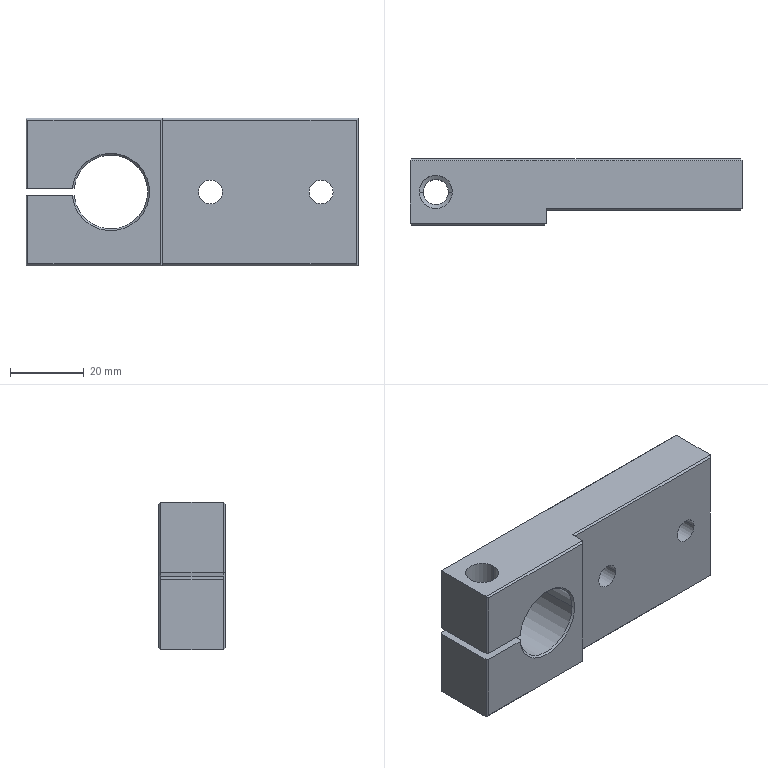Part | NX | 1 solid | 45 faces | box 90 x 18 x 40 mm | volume 46471 mm3 | plane 26 | cylinder 14 | cone 5 | commonest cylinder face diameters 6.5 x4 11 x4 6.8 x2 9 x2 20 x2
STEP:
#1=CARTESIAN_POINT('',(0.,17.5,-15.));
#2=VERTEX_POINT('',#1);
#3=CARTESIAN_POINT('',(0.5,18.,-14.5));
#4=VERTEX_POINT('',#3);
#5=CARTESIAN_POINT('',(15.,32.5,0.));
#6=DIRECTION('',(0.5774,0.5774,0.5774));
#7=VECTOR('',#6,1000.);
#8=LINE('',#5,#7);
#9=EDGE_CURVE('',#2,#4,#8,.T.);
#10=ORIENTED_EDGE('',*,*,#9,.F.);
#11=CARTESIAN_POINT('',(0.,17.5,4.));
#12=VERTEX_POINT('',#11);
#13=CARTESIAN_POINT('',(0.,17.5,0.));
#14=DIRECTION('',(0.,0.,-1.));
#15=VECTOR('',#14,1000.);
#16=LINE('',#13,#15);
#17=EDGE_CURVE('',#12,#2,#16,.T.);
#18=ORIENTED_EDGE('',*,*,#17,.F.);
#19=CARTESIAN_POINT('',(0.5,18.,4.));
#20=VERTEX_POINT('',#19);
#21=CARTESIAN_POINT('',(-17.5,0.,4.));
#22=DIRECTION('',(0.7071,0.7071,0.));
#23=VECTOR('',#22,1000.);
#24=LINE('',#21,#23);
#25=EDGE_CURVE('',#12,#20,#24,.T.);
#26=ORIENTED_EDGE('',*,*,#25,.T.);
#27=CARTESIAN_POINT('',(0.5,18.,0.));
#28=DIRECTION('',(0.,0.,-1.));
#29=VECTOR('',#28,1000.);
#30=LINE('',#27,#29);
#31=EDGE_CURVE('',#20,#4,#30,.T.);
#32=ORIENTED_EDGE('',*,*,#31,.T.);
#33=EDGE_LOOP('',(#10,#18,#26,#32));
#34=FACE_BOUND('',#33,.T.);
#35=CARTESIAN_POINT('',(0.,17.5,-16.5));
#36=DIRECTION('',(-0.7071,0.7071,0.));
#37=DIRECTION('',(0.,0.,1.));
#38=AXIS2_PLACEMENT_3D('',#35,#36,#37);
#39=PLANE('',#38);
#40=ADVANCED_FACE('',(#34),#39,.T.);
#41=CARTESIAN_POINT('',(37.,0.5,-15.));
#42=VERTEX_POINT('',#41);
#43=CARTESIAN_POINT('',(36.5,0.,-14.5));
#44=VERTEX_POINT('',#43);
#45=CARTESIAN_POINT('',(22.,-14.5,0.));
#46=DIRECTION('',(-0.5774,-0.5774,0.5774));
#47=VECTOR('',#46,1000.);
#48=LINE('',#45,#47);
#49=EDGE_CURVE('',#42,#44,#48,.T.);
#50=ORIENTED_EDGE('',*,*,#49,.T.);
#51=CARTESIAN_POINT('',(0.5,0.,-14.5));
#52=VERTEX_POINT('',#51);
#53=CARTESIAN_POINT('',(0.,0.,-14.5));
#54=DIRECTION('',(-1.,0.,0.));
#55=VECTOR('',#54,1000.);
#56=LINE('',#53,#55);
#57=EDGE_CURVE('',#44,#52,#56,.T.);
#58=ORIENTED_EDGE('',*,*,#57,.T.);
#59=CARTESIAN_POINT('',(0.,0.5,-15.));
#60=VERTEX_POINT('',#59);
#61=CARTESIAN_POINT('',(15.,-14.5,0.));
#62=DIRECTION('',(0.5774,-0.5774,0.5774));
#63=VECTOR('',#62,1000.);
#64=LINE('',#61,#63);
#65=EDGE_CURVE('',#60,#52,#64,.T.);
#66=ORIENTED_EDGE('',*,*,#65,.F.);
#67=CARTESIAN_POINT('',(0.,0.5,-15.));
#68=DIRECTION('',(1.,0.,0.));
#69=VECTOR('',#68,1000.);
#70=LINE('',#67,#69);
#71=EDGE_CURVE('',#60,#42,#70,.T.);
#72=ORIENTED_EDGE('',*,*,#71,.T.);
#73=EDGE_LOOP('',(#50,#58,#66,#72));
#74=FACE_BOUND('',#73,.T.);
#75=CARTESIAN_POINT('',(1.,0.5,-15.));
#76=DIRECTION('',(0.,-0.7071,-0.7071));
#77=DIRECTION('',(0.,-0.7071,0.7071));
#78=AXIS2_PLACEMENT_3D('',#75,#76,#77);
#79=PLANE('',#78);
#80=ADVANCED_FACE('',(#74),#79,.T.);
#81=CARTESIAN_POINT('',(37.,4.,24.5));
#82=VERTEX_POINT('',#81);
#83=CARTESIAN_POINT('',(37.,4.,-14.5));
#84=VERTEX_POINT('',#83);
#85=CARTESIAN_POINT('',(37.,4.,0.));
#86=DIRECTION('',(0.,0.,-1.));
#87=VECTOR('',#86,1000.);
#88=LINE('',#85,#87);
#89=EDGE_CURVE('',#82,#84,#88,.T.);
#90=ORIENTED_EDGE('',*,*,#89,.F.);
#91=CARTESIAN_POINT('',(37.,4.5,25.));
#92=VERTEX_POINT('',#91);
#93=CARTESIAN_POINT('',(37.,-20.5,0.));
#94=DIRECTION('',(0.,-0.7071,-0.7071));
#95=VECTOR('',#94,1000.);
#96=LINE('',#93,#95);
#97=EDGE_CURVE('',#92,#82,#96,.T.);
#98=ORIENTED_EDGE('',*,*,#97,.F.);
#99=CARTESIAN_POINT('',(37.,0.5,25.));
#100=VERTEX_POINT('',#99);
#101=CARTESIAN_POINT('',(37.,0.,25.));
#102=DIRECTION('',(0.,1.,0.));
#103=VECTOR('',#102,1000.);
#104=LINE('',#101,#103);
#105=EDGE_CURVE('',#100,#92,#104,.T.);
#106=ORIENTED_EDGE('',*,*,#105,.F.);
#107=CARTESIAN_POINT('',(37.,0.5,0.));
#108=DIRECTION('',(0.,0.,1.));
#109=VECTOR('',#108,1000.);
#110=LINE('',#107,#109);
#111=EDGE_CURVE('',#42,#100,#110,.T.);
#112=ORIENTED_EDGE('',*,*,#111,.F.);
#113=CARTESIAN_POINT('',(37.,4.5,-15.));
#114=VERTEX_POINT('',#113);
#115=CARTESIAN_POINT('',(37.,0.,-15.));
#116=DIRECTION('',(0.,1.,0.));
#117=VECTOR('',#116,1000.);
#118=LINE('',#115,#117);
#119=EDGE_CURVE('',#42,#114,#118,.T.);
#120=ORIENTED_EDGE('',*,*,#119,.T.);
#121=CARTESIAN_POINT('',(37.,-10.5,0.));
#122=DIRECTION('',(0.,-0.7071,0.7071));
#123=VECTOR('',#122,1000.);
#124=LINE('',#121,#123);
#125=EDGE_CURVE('',#114,#84,#124,.T.);
#126=ORIENTED_EDGE('',*,*,#125,.T.);
#127=EDGE_LOOP('',(#90,#98,#106,#112,#120,#126));
#128=FACE_BOUND('',#127,.T.);
#129=CARTESIAN_POINT('',(37.,0.,-17.5));
#130=DIRECTION('',(1.,0.,0.));
#131=DIRECTION('',(0.,1.,0.));
#132=AXIS2_PLACEMENT_3D('',#129,#130,#131);
#133=PLANE('',#132);
#134=ADVANCED_FACE('',(#128),#133,.T.);
#135=CARTESIAN_POINT('',(44.5,11.5,5.));
#136=VERTEX_POINT('',#135);
#137=CARTESIAN_POINT('',(55.5,11.5,5.));
#138=VERTEX_POINT('',#137);
#139=CARTESIAN_POINT('',(50.,11.5,5.));
#140=DIRECTION('',(0.,1.,0.));
#141=DIRECTION('',(1.,0.,0.));
#142=AXIS2_PLACEMENT_3D('',#139,#140,#141);
#143=CIRCLE('',#142,5.5);
#144=EDGE_CURVE('',#136,#138,#143,.T.);
#145=ORIENTED_EDGE('',*,*,#144,.T.);
#146=CARTESIAN_POINT('',(50.,11.5,5.));
#147=DIRECTION('',(0.,1.,0.));
#148=DIRECTION('',(1.,0.,0.));
#149=AXIS2_PLACEMENT_3D('',#146,#147,#148);
#150=CIRCLE('',#149,5.5);
#151=EDGE_CURVE('',#138,#136,#150,.T.);
#152=ORIENTED_EDGE('',*,*,#151,.T.);
#153=EDGE_LOOP('',(#145,#152));
#154=FACE_BOUND('',#153,.T.);
#155=CARTESIAN_POINT('',(53.25,11.5,5.));
#156=VERTEX_POINT('',#155);
#157=CARTESIAN_POINT('',(46.75,11.5,5.));
#158=VERTEX_POINT('',#157);
#159=CARTESIAN_POINT('',(50.,11.5,5.));
#160=DIRECTION('',(0.,1.,0.));
#161=DIRECTION('',(1.,0.,0.));
#162=AXIS2_PLACEMENT_3D('',#159,#160,#161);
#163=CIRCLE('',#162,3.25);
#164=EDGE_CURVE('',#156,#158,#163,.T.);
#165=ORIENTED_EDGE('',*,*,#164,.F.);
#166=CARTESIAN_POINT('',(50.,11.5,5.));
#167=DIRECTION('',(0.,1.,0.));
#168=DIRECTION('',(1.,0.,0.));
#169=AXIS2_PLACEMENT_3D('',#166,#167,#168);
#170=CIRCLE('',#169,3.25);
#171=EDGE_CURVE('',#158,#156,#170,.T.);
#172=ORIENTED_EDGE('',*,*,#171,.F.);
#173=EDGE_LOOP('',(#165,#172));
#174=FACE_BOUND('',#173,.T.);
#175=CARTESIAN_POINT('',(50.,11.5,5.));
#176=DIRECTION('',(0.,1.,0.));
#177=DIRECTION('',(1.,0.,0.));
#178=AXIS2_PLACEMENT_3D('',#175,#176,#177);
#179=PLANE('',#178);
#180=ADVANCED_FACE('',(#154,#174),#179,.T.);
#181=CARTESIAN_POINT('',(74.5,11.5,5.));
#182=VERTEX_POINT('',#181);
#183=CARTESIAN_POINT('',(85.5,11.5,5.));
#184=VERTEX_POINT('',#183);
#185=CARTESIAN_POINT('',(80.,11.5,5.));
#186=DIRECTION('',(0.,1.,0.));
#187=DIRECTION('',(1.,0.,0.));
#188=AXIS2_PLACEMENT_3D('',#185,#186,#187);
#189=CIRCLE('',#188,5.5);
#190=EDGE_CURVE('',#182,#184,#189,.T.);
#191=ORIENTED_EDGE('',*,*,#190,.F.);
#192=CARTESIAN_POINT('',(74.5,18.,5.));
#193=VERTEX_POINT('',#192);
#194=CARTESIAN_POINT('',(74.5,-2.79,5.));
#195=DIRECTION('',(0.,1.,0.));
#196=VECTOR('',#195,1000.);
#197=LINE('',#194,#196);
#198=EDGE_CURVE('',#182,#193,#197,.T.);
#199=ORIENTED_EDGE('',*,*,#198,.T.);
#200=CARTESIAN_POINT('',(85.5,18.,5.));
#201=VERTEX_POINT('',#200);
#202=CARTESIAN_POINT('',(80.,18.,5.));
#203=DIRECTION('',(0.,1.,0.));
#204=DIRECTION('',(1.,0.,0.));
#205=AXIS2_PLACEMENT_3D('',#202,#203,#204);
#206=CIRCLE('',#205,5.5);
#207=EDGE_CURVE('',#193,#201,#206,.T.);
#208=ORIENTED_EDGE('',*,*,#207,.T.);
#209=CARTESIAN_POINT('',(85.5,-2.79,5.));
#210=DIRECTION('',(0.,1.,0.));
#211=VECTOR('',#210,1000.);
#212=LINE('',#209,#211);
#213=EDGE_CURVE('',#184,#201,#212,.T.);
#214=ORIENTED_EDGE('',*,*,#213,.F.);
#215=EDGE_LOOP('',(#191,#199,#208,#214));
#216=FACE_BOUND('',#215,.T.);
#217=CARTESIAN_POINT('',(80.,-2.79,5.));
#218=DIRECTION('',(0.,1.,0.));
#219=DIRECTION('',(1.,0.,0.));
#220=AXIS2_PLACEMENT_3D('',#217,#218,#219);
#221=CYLINDRICAL_SURFACE('',#220,5.5);
#222=ADVANCED_FACE('',(#216),#221,.F.);
#223=CARTESIAN_POINT('',(89.5,18.,24.5));
#224=VERTEX_POINT('',#223);
#225=CARTESIAN_POINT('',(90.,17.5,25.));
#226=VERTEX_POINT('',#225);
#227=CARTESIAN_POINT('',(65.,42.5,0.));
#228=DIRECTION('',(0.5774,-0.5774,0.5774));
#229=VECTOR('',#228,1000.);
#230=LINE('',#227,#229);
#231=EDGE_CURVE('',#224,#226,#230,.T.);
#232=ORIENTED_EDGE('',*,*,#231,.T.);
#233=CARTESIAN_POINT('',(90.,17.5,-15.));
#234=VERTEX_POINT('',#233);
#235=CARTESIAN_POINT('',(90.,17.5,0.));
#236=DIRECTION('',(0.,0.,1.));
#237=VECTOR('',#236,1000.);
#238=LINE('',#235,#237);
#239=EDGE_CURVE('',#234,#226,#238,.T.);
#240=ORIENTED_EDGE('',*,*,#239,.F.);
#241=CARTESIAN_POINT('',(89.5,18.,-14.5));
#242=VERTEX_POINT('',#241);
#243=CARTESIAN_POINT('',(75.,32.5,0.));
#244=DIRECTION('',(0.5774,-0.5774,-0.5774));
#245=VECTOR('',#244,1000.);
#246=LINE('',#243,#245);
#247=EDGE_CURVE('',#242,#234,#246,.T.);
#248=ORIENTED_EDGE('',*,*,#247,.F.);
#249=CARTESIAN_POINT('',(89.5,18.,0.));
#250=DIRECTION('',(0.,0.,-1.));
#251=VECTOR('',#250,1000.);
#252=LINE('',#249,#251);
#253=EDGE_CURVE('',#224,#242,#252,.T.);
#254=ORIENTED_EDGE('',*,*,#253,.F.);
#255=EDGE_LOOP('',(#232,#240,#248,#254));
#256=FACE_BOUND('',#255,.T.);
#257=CARTESIAN_POINT('',(89.5,18.,-16.5));
#258=DIRECTION('',(0.7071,0.7071,0.));
#259=DIRECTION('',(0.,0.,-1.));
#260=AXIS2_PLACEMENT_3D('',#257,#258,#259);
#261=PLANE('',#260);
#262=ADVANCED_FACE('',(#256),#261,.T.);
#263=CARTESIAN_POINT('',(10.4,9.,-15.));
#264=VERTEX_POINT('',#263);
#265=CARTESIAN_POINT('',(3.6,9.,-15.));
#266=VERTEX_POINT('',#265);
#267=CARTESIAN_POINT('',(7.,9.,-15.));
#268=DIRECTION('',(0.,0.,1.));
#269=DIRECTION('',(1.,0.,0.));
#270=AXIS2_PLACEMENT_3D('',#267,#268,#269);
#271=CIRCLE('',#270,3.4);
#272=EDGE_CURVE('',#264,#266,#271,.T.);
#273=ORIENTED_EDGE('',*,*,#272,.F.);
#274=CARTESIAN_POINT('',(10.4,9.,3.329));
#275=VERTEX_POINT('',#274);
#276=CARTESIAN_POINT('',(10.4,9.,4.));
#277=DIRECTION('',(0.,0.,1.));
#278=VECTOR('',#277,1000.);
#279=LINE('',#276,#278);
#280=EDGE_CURVE('',#264,#275,#279,.T.);
#281=ORIENTED_EDGE('',*,*,#280,.T.);
#282=CARTESIAN_POINT('',(3.6,9.,3.329));
#283=VERTEX_POINT('',#282);
#284=CARTESIAN_POINT('',(7.,9.,3.329));
#285=DIRECTION('',(0.,0.,1.));
#286=DIRECTION('',(1.,0.,0.));
#287=AXIS2_PLACEMENT_3D('',#284,#285,#286);
#288=CIRCLE('',#287,3.4);
#289=EDGE_CURVE('',#275,#283,#288,.T.);
#290=ORIENTED_EDGE('',*,*,#289,.T.);
#291=CARTESIAN_POINT('',(3.6,9.,4.));
#292=DIRECTION('',(0.,0.,1.));
#293=VECTOR('',#292,1000.);
#294=LINE('',#291,#293);
#295=EDGE_CURVE('',#266,#283,#294,.T.);
#296=ORIENTED_EDGE('',*,*,#295,.F.);
#297=EDGE_LOOP('',(#273,#281,#290,#296));
#298=FACE_BOUND('',#297,.T.);
#299=CARTESIAN_POINT('',(7.,9.,4.));
#300=DIRECTION('',(0.,0.,1.));
#301=DIRECTION('',(1.,0.,0.));
#302=AXIS2_PLACEMENT_3D('',#299,#300,#301);
#303=CYLINDRICAL_SURFACE('',#302,3.4);
#304=ADVANCED_FACE('',(#298),#303,.F.);
#305=CARTESIAN_POINT('',(76.75,4.,5.));
#306=VERTEX_POINT('',#305);
#307=CARTESIAN_POINT('',(83.25,4.,5.));
#308=VERTEX_POINT('',#307);
#309=CARTESIAN_POINT('',(80.,4.,5.));
#310=DIRECTION('',(0.,1.,0.));
#311=DIRECTION('',(1.,0.,0.));
#312=AXIS2_PLACEMENT_3D('',#309,#310,#311);
#313=CIRCLE('',#312,3.25);
#314=EDGE_CURVE('',#306,#308,#313,.T.);
#315=ORIENTED_EDGE('',*,*,#314,.F.);
#316=CARTESIAN_POINT('',(76.75,11.5,5.));
#317=VERTEX_POINT('',#316);
#318=CARTESIAN_POINT('',(76.75,-2.79,5.));
#319=DIRECTION('',(0.,1.,0.));
#320=VECTOR('',#319,1000.);
#321=LINE('',#318,#320);
#322=EDGE_CURVE('',#306,#317,#321,.T.);
#323=ORIENTED_EDGE('',*,*,#322,.T.);
#324=CARTESIAN_POINT('',(83.25,11.5,5.));
#325=VERTEX_POINT('',#324);
#326=CARTESIAN_POINT('',(80.,11.5,5.));
#327=DIRECTION('',(0.,1.,0.));
#328=DIRECTION('',(1.,0.,0.));
#329=AXIS2_PLACEMENT_3D('',#326,#327,#328);
#330=CIRCLE('',#329,3.25);
#331=EDGE_CURVE('',#317,#325,#330,.T.);
#332=ORIENTED_EDGE('',*,*,#331,.T.);
#333=CARTESIAN_POINT('',(83.25,-2.79,5.));
#334=DIRECTION('',(0.,1.,0.));
#335=VECTOR('',#334,1000.);
#336=LINE('',#333,#335);
#337=EDGE_CURVE('',#308,#325,#336,.T.);
#338=ORIENTED_EDGE('',*,*,#337,.F.);
#339=EDGE_LOOP('',(#315,#323,#332,#338));
#340=FACE_BOUND('',#339,.T.);
#341=CARTESIAN_POINT('',(80.,-2.79,5.));
#342=DIRECTION('',(0.,1.,0.));
#343=DIRECTION('',(1.,0.,0.));
#344=AXIS2_PLACEMENT_3D('',#341,#342,#343);
#345=CYLINDRICAL_SURFACE('',#344,3.25);
#346=ADVANCED_FACE('',(#340),#345,.F.);
#347=CARTESIAN_POINT('',(44.5,18.,5.));
#348=VERTEX_POINT('',#347);
#349=CARTESIAN_POINT('',(55.5,18.,5.));
#350=VERTEX_POINT('',#349);
#351=CARTESIAN_POINT('',(50.,18.,5.));
#352=DIRECTION('',(0.,1.,0.));
#353=DIRECTION('',(1.,0.,0.));
#354=AXIS2_PLACEMENT_3D('',#351,#352,#353);
#355=CIRCLE('',#354,5.5);
#356=EDGE_CURVE('',#348,#350,#355,.T.);
#357=ORIENTED_EDGE('',*,*,#356,.T.);
#358=CARTESIAN_POINT('',(55.5,-2.79,5.));
#359=DIRECTION('',(0.,1.,0.));
#360=VECTOR('',#359,1000.);
#361=LINE('',#358,#360);
#362=EDGE_CURVE('',#138,#350,#361,.T.);
#363=ORIENTED_EDGE('',*,*,#362,.F.);
#364=ORIENTED_EDGE('',*,*,#144,.F.);
#365=CARTESIAN_POINT('',(44.5,-2.79,5.));
#366=DIRECTION('',(0.,1.,0.));
#367=VECTOR('',#366,1000.);
#368=LINE('',#365,#367);
#369=EDGE_CURVE('',#136,#348,#368,.T.);
#370=ORIENTED_EDGE('',*,*,#369,.T.);
#371=EDGE_LOOP('',(#357,#363,#364,#370));
#372=FACE_BOUND('',#371,.T.);
#373=CARTESIAN_POINT('',(50.,-2.79,5.));
#374=DIRECTION('',(0.,1.,0.));
#375=DIRECTION('',(1.,0.,0.));
#376=AXIS2_PLACEMENT_3D('',#373,#374,#375);
#377=CYLINDRICAL_SURFACE('',#376,5.5);
#378=ADVANCED_FACE('',(#372),#377,.F.);
#379=CARTESIAN_POINT('',(90.,4.5,-15.));
#380=VERTEX_POINT('',#379);
#381=CARTESIAN_POINT('',(89.5,4.,-14.5));
#382=VERTEX_POINT('',#381);
#383=CARTESIAN_POINT('',(75.,-10.5,0.));
#384=DIRECTION('',(-0.5774,-0.5774,0.5774));
#385=VECTOR('',#384,1000.);
#386=LINE('',#383,#385);
#387=EDGE_CURVE('',#380,#382,#386,.T.);
#388=ORIENTED_EDGE('',*,*,#387,.T.);
#389=CARTESIAN_POINT('',(0.,4.,-14.5));
#390=DIRECTION('',(-1.,0.,0.));
#391=VECTOR('',#390,1000.);
#392=LINE('',#389,#391);
#393=EDGE_CURVE('',#382,#84,#392,.T.);
#394=ORIENTED_EDGE('',*,*,#393,.T.);
#395=ORIENTED_EDGE('',*,*,#125,.F.);
#396=CARTESIAN_POINT('',(0.,4.5,-15.));
#397=DIRECTION('',(1.,0.,0.));
#398=VECTOR('',#397,1000.);
#399=LINE('',#396,#398);
#400=EDGE_CURVE('',#114,#380,#399,.T.);
#401=ORIENTED_EDGE('',*,*,#400,.T.);
#402=EDGE_LOOP('',(#388,#394,#395,#401));
#403=FACE_BOUND('',#402,.T.);
#404=CARTESIAN_POINT('',(37.,4.5,-15.));
#405=DIRECTION('',(0.,-0.7071,-0.7071));
#406=DIRECTION('',(0.,-0.7071,0.7071));
#407=AXIS2_PLACEMENT_3D('',#404,#405,#406);
#408=PLANE('',#407);
#409=ADVANCED_FACE('',(#403),#408,.T.);
#410=CARTESIAN_POINT('',(0.5,0.,24.5));
#411=VERTEX_POINT('',#410);
#412=CARTESIAN_POINT('',(0.,0.5,25.));
#413=VERTEX_POINT('',#412);
#414=CARTESIAN_POINT('',(25.,-24.5,0.));
#415=DIRECTION('',(-0.5774,0.5774,0.5774));
#416=VECTOR('',#415,1000.);
#417=LINE('',#414,#416);
#418=EDGE_CURVE('',#411,#413,#417,.T.);
#419=ORIENTED_EDGE('',*,*,#418,.T.);
#420=CARTESIAN_POINT('',(0.,0.5,6.));
#421=VERTEX_POINT('',#420);
#422=CARTESIAN_POINT('',(0.,0.5,0.));
#423=DIRECTION('',(0.,0.,1.));
#424=VECTOR('',#423,1000.);
#425=LINE('',#422,#424);
#426=EDGE_CURVE('',#421,#413,#425,.T.);
#427=ORIENTED_EDGE('',*,*,#426,.F.);
#428=CARTESIAN_POINT('',(0.5,0.,6.));
#429=VERTEX_POINT('',#428);
#430=CARTESIAN_POINT('',(0.5,0.,6.));
#431=DIRECTION('',(0.7071,-0.7071,0.));
#432=VECTOR('',#431,1000.);
#433=LINE('',#430,#432);
#434=EDGE_CURVE('',#421,#429,#433,.T.);
#435=ORIENTED_EDGE('',*,*,#434,.T.);
#436=CARTESIAN_POINT('',(0.5,0.,0.));
#437=DIRECTION('',(0.,0.,-1.));
#438=VECTOR('',#437,1000.);
#439=LINE('',#436,#438);
#440=EDGE_CURVE('',#411,#429,#439,.T.);
#441=ORIENTED_EDGE('',*,*,#440,.F.);
#442=EDGE_LOOP('',(#419,#427,#435,#441));
#443=FACE_BOUND('',#442,.T.);
#444=CARTESIAN_POINT('',(0.5,0.,6.));
#445=DIRECTION('',(-0.7071,-0.7071,0.));
#446=DIRECTION('',(-0.7071,0.7071,0.));
#447=AXIS2_PLACEMENT_3D('',#444,#445,#446);
#448=PLANE('',#447);
#449=ADVANCED_FACE('',(#443),#448,.T.);
#450=ORIENTED_EDGE('',*,*,#111,.T.);
#451=CARTESIAN_POINT('',(36.5,0.,24.5));
#452=VERTEX_POINT('',#451);
#453=CARTESIAN_POINT('',(12.,-24.5,0.));
#454=DIRECTION('',(-0.5774,-0.5774,-0.5774));
#455=VECTOR('',#454,1000.);
#456=LINE('',#453,#455);
#457=EDGE_CURVE('',#100,#452,#456,.T.);
#458=ORIENTED_EDGE('',*,*,#457,.T.);
#459=CARTESIAN_POINT('',(36.5,0.,0.));
#460=DIRECTION('',(0.,0.,1.));
#461=VECTOR('',#460,1000.);
#462=LINE('',#459,#461);
#463=EDGE_CURVE('',#44,#452,#462,.T.);
#464=ORIENTED_EDGE('',*,*,#463,.F.);
#465=ORIENTED_EDGE('',*,*,#49,.F.);
#466=EDGE_LOOP('',(#450,#458,#464,#465));
#467=FACE_BOUND('',#466,.T.);
#468=CARTESIAN_POINT('',(37.,0.5,-17.));
#469=DIRECTION('',(0.7071,-0.7071,0.));
#470=DIRECTION('',(0.,0.,-1.));
#471=AXIS2_PLACEMENT_3D('',#468,#469,#470);
#472=PLANE('',#471);
#473=ADVANCED_FACE('',(#467),#472,.T.);
#474=CARTESIAN_POINT('',(12.548,0.,6.));
#475=VERTEX_POINT('',#474);
#476=CARTESIAN_POINT('',(0.,0.,6.));
#477=DIRECTION('',(1.,0.,0.));
#478=VECTOR('',#477,1000.);
#479=LINE('',#476,#478);
#480=EDGE_CURVE('',#429,#475,#479,.T.);
#481=ORIENTED_EDGE('',*,*,#480,.F.);
#482=ORIENTED_EDGE('',*,*,#434,.F.);
#483=CARTESIAN_POINT('',(0.,17.5,6.));
#484=VERTEX_POINT('',#483);
#485=CARTESIAN_POINT('',(0.,0.,6.));
#486=DIRECTION('',(0.,-1.,0.));
#487=VECTOR('',#486,1000.);
#488=LINE('',#485,#487);
#489=EDGE_CURVE('',#484,#421,#488,.T.);
#490=ORIENTED_EDGE('',*,*,#489,.F.);
#491=CARTESIAN_POINT('',(0.5,18.,6.));
#492=VERTEX_POINT('',#491);
#493=CARTESIAN_POINT('',(-17.5,0.,6.));
#494=DIRECTION('',(-0.7071,-0.7071,0.));
#495=VECTOR('',#494,1000.);
#496=LINE('',#493,#495);
#497=EDGE_CURVE('',#492,#484,#496,.T.);
#498=ORIENTED_EDGE('',*,*,#497,.F.);
#499=CARTESIAN_POINT('',(12.548,18.,6.));
#500=VERTEX_POINT('',#499);
#501=CARTESIAN_POINT('',(0.,18.,6.));
#502=DIRECTION('',(-1.,0.,0.));
#503=VECTOR('',#502,1000.);
#504=LINE('',#501,#503);
#505=EDGE_CURVE('',#500,#492,#504,.T.);
#506=ORIENTED_EDGE('',*,*,#505,.F.);
#507=CARTESIAN_POINT('',(13.05,17.5,6.));
#508=VERTEX_POINT('',#507);
#509=CARTESIAN_POINT('',(12.548,18.,6.));
#510=CARTESIAN_POINT('',(12.604,17.944,6.));
#511=CARTESIAN_POINT('',(12.715,17.833,6.));
#512=CARTESIAN_POINT('',(12.883,17.667,6.));
#513=CARTESIAN_POINT('',(12.994,17.556,6.));
#514=CARTESIAN_POINT('',(13.05,17.5,6.));
#515=B_SPLINE_CURVE_WITH_KNOTS('',3,(#509,#510,#511,#512,#513,#514),.UNSPECIFIED.,.F.,.F.,(4,1,1,4),(0.,0.3333,0.6667,1.),.UNSPECIFIED.);
#516=EDGE_CURVE('',#500,#508,#515,.T.);
#517=ORIENTED_EDGE('',*,*,#516,.T.);
#518=CARTESIAN_POINT('',(13.05,0.5,6.));
#519=VERTEX_POINT('',#518);
#520=CARTESIAN_POINT('',(13.05,17.5,6.));
#521=DIRECTION('',(0.,-1.,0.));
#522=VECTOR('',#521,1000.);
#523=LINE('',#520,#522);
#524=EDGE_CURVE('',#508,#519,#523,.T.);
#525=ORIENTED_EDGE('',*,*,#524,.T.);
#526=CARTESIAN_POINT('',(13.05,0.5,6.));
#527=CARTESIAN_POINT('',(12.994,0.4444,6.));
#528=CARTESIAN_POINT('',(12.883,0.3333,6.));
#529=CARTESIAN_POINT('',(12.715,0.1667,6.));
#530=CARTESIAN_POINT('',(12.604,0.05556,6.));
#531=CARTESIAN_POINT('',(12.548,0.,6.));
#532=B_SPLINE_CURVE_WITH_KNOTS('',3,(#526,#527,#528,#529,#530,#531),.UNSPECIFIED.,.F.,.F.,(4,1,1,4),(0.,0.3333,0.6667,1.),.UNSPECIFIED.);
#533=EDGE_CURVE('',#519,#475,#532,.T.);
#534=ORIENTED_EDGE('',*,*,#533,.T.);
#535=EDGE_LOOP('',(#481,#482,#490,#498,#506,#517,#525,#534));
#536=FACE_BOUND('',#535,.T.);
#537=CARTESIAN_POINT('',(2.5,9.,6.));
#538=VERTEX_POINT('',#537);
#539=CARTESIAN_POINT('',(11.5,9.,6.));
#540=VERTEX_POINT('',#539);
#541=CARTESIAN_POINT('',(7.,9.,6.));
#542=DIRECTION('',(0.,0.,-1.));
#543=DIRECTION('',(-1.,0.,0.));
#544=AXIS2_PLACEMENT_3D('',#541,#542,#543);
#545=CIRCLE('',#544,4.5);
#546=EDGE_CURVE('',#538,#540,#545,.T.);
#547=ORIENTED_EDGE('',*,*,#546,.F.);
#548=CARTESIAN_POINT('',(7.,9.,6.));
#549=DIRECTION('',(0.,0.,-1.));
#550=DIRECTION('',(-1.,0.,0.));
#551=AXIS2_PLACEMENT_3D('',#548,#549,#550);
#552=CIRCLE('',#551,4.5);
#553=EDGE_CURVE('',#540,#538,#552,.T.);
#554=ORIENTED_EDGE('',*,*,#553,.F.);
#555=EDGE_LOOP('',(#547,#554));
#556=FACE_BOUND('',#555,.T.);
#557=CARTESIAN_POINT('',(0.,18.,6.));
#558=DIRECTION('',(0.,0.,1.));
#559=DIRECTION('',(1.,0.,0.));
#560=AXIS2_PLACEMENT_3D('',#557,#558,#559);
#561=PLANE('',#560);
#562=ADVANCED_FACE('',(#536,#556),#561,.F.);
#563=CARTESIAN_POINT('',(89.5,4.,24.5));
#564=VERTEX_POINT('',#563);
#565=CARTESIAN_POINT('',(89.5,4.,0.));
#566=DIRECTION('',(0.,0.,1.));
#567=VECTOR('',#566,1000.);
#568=LINE('',#565,#567);
#569=EDGE_CURVE('',#382,#564,#568,.T.);
#570=ORIENTED_EDGE('',*,*,#569,.T.);
#571=CARTESIAN_POINT('',(0.,4.,24.5));
#572=DIRECTION('',(-1.,0.,0.));
#573=VECTOR('',#572,1000.);
#574=LINE('',#571,#573);
#575=EDGE_CURVE('',#564,#82,#574,.T.);
#576=ORIENTED_EDGE('',*,*,#575,.T.);
#577=ORIENTED_EDGE('',*,*,#89,.T.);
#578=ORIENTED_EDGE('',*,*,#393,.F.);
#579=EDGE_LOOP('',(#570,#576,#577,#578));
#580=FACE_BOUND('',#579,.T.);
#581=ORIENTED_EDGE('',*,*,#314,.T.);
#582=CARTESIAN_POINT('',(80.,4.,5.));
#583=DIRECTION('',(0.,1.,0.));
#584=DIRECTION('',(1.,0.,0.));
#585=AXIS2_PLACEMENT_3D('',#582,#583,#584);
#586=CIRCLE('',#585,3.25);
#587=EDGE_CURVE('',#308,#306,#586,.T.);
#588=ORIENTED_EDGE('',*,*,#587,.T.);
#589=EDGE_LOOP('',(#581,#588));
#590=FACE_BOUND('',#589,.T.);
#591=CARTESIAN_POINT('',(46.75,4.,5.));
#592=VERTEX_POINT('',#591);
#593=CARTESIAN_POINT('',(53.25,4.,5.));
#594=VERTEX_POINT('',#593);
#595=CARTESIAN_POINT('',(50.,4.,5.));
#596=DIRECTION('',(0.,1.,0.));
#597=DIRECTION('',(1.,0.,0.));
#598=AXIS2_PLACEMENT_3D('',#595,#596,#597);
#599=CIRCLE('',#598,3.25);
#600=EDGE_CURVE('',#592,#594,#599,.T.);
#601=ORIENTED_EDGE('',*,*,#600,.T.);
#602=CARTESIAN_POINT('',(50.,4.,5.));
#603=DIRECTION('',(0.,1.,0.));
#604=DIRECTION('',(1.,0.,0.));
#605=AXIS2_PLACEMENT_3D('',#602,#603,#604);
#606=CIRCLE('',#605,3.25);
#607=EDGE_CURVE('',#594,#592,#606,.T.);
#608=ORIENTED_EDGE('',*,*,#607,.T.);
#609=EDGE_LOOP('',(#601,#608));
#610=FACE_BOUND('',#609,.T.);
#611=CARTESIAN_POINT('',(37.,4.,-17.5));
#612=DIRECTION('',(0.,-1.,0.));
#613=DIRECTION('',(0.,0.,-1.));
#614=AXIS2_PLACEMENT_3D('',#611,#612,#613);
#615=PLANE('',#614);
#616=ADVANCED_FACE('',(#580,#590,#610),#615,.T.);
#617=ORIENTED_EDGE('',*,*,#31,.F.);
#618=CARTESIAN_POINT('',(12.548,18.,4.));
#619=VERTEX_POINT('',#618);
#620=CARTESIAN_POINT('',(0.,18.,4.));
#621=DIRECTION('',(1.,0.,0.));
#622=VECTOR('',#621,1000.);
#623=LINE('',#620,#622);
#624=EDGE_CURVE('',#20,#619,#623,.T.);
#625=ORIENTED_EDGE('',*,*,#624,.T.);
#626=CARTESIAN_POINT('',(33.5,18.,5.));
#627=VERTEX_POINT('',#626);
#628=CARTESIAN_POINT('',(23.,18.,5.));
#629=DIRECTION('',(0.,1.,0.));
#630=DIRECTION('',(1.,0.,0.));
#631=AXIS2_PLACEMENT_3D('',#628,#629,#630);
#632=CIRCLE('',#631,10.5);
#633=EDGE_CURVE('',#627,#619,#632,.T.);
#634=ORIENTED_EDGE('',*,*,#633,.F.);
#635=CARTESIAN_POINT('',(23.,18.,5.));
#636=DIRECTION('',(0.,1.,0.));
#637=DIRECTION('',(1.,0.,0.));
#638=AXIS2_PLACEMENT_3D('',#635,#636,#637);
#639=CIRCLE('',#638,10.5);
#640=EDGE_CURVE('',#500,#627,#639,.T.);
#641=ORIENTED_EDGE('',*,*,#640,.F.);
#642=ORIENTED_EDGE('',*,*,#505,.T.);
#643=CARTESIAN_POINT('',(0.5,18.,24.5));
#644=VERTEX_POINT('',#643);
#645=CARTESIAN_POINT('',(0.5,18.,0.));
#646=DIRECTION('',(0.,0.,1.));
#647=VECTOR('',#646,1000.);
#648=LINE('',#645,#647);
#649=EDGE_CURVE('',#492,#644,#648,.T.);
#650=ORIENTED_EDGE('',*,*,#649,.T.);
#651=CARTESIAN_POINT('',(0.,18.,24.5));
#652=DIRECTION('',(1.,0.,0.));
#653=VECTOR('',#652,1000.);
#654=LINE('',#651,#653);
#655=EDGE_CURVE('',#644,#224,#654,.T.);
#656=ORIENTED_EDGE('',*,*,#655,.T.);
#657=ORIENTED_EDGE('',*,*,#253,.T.);
#658=CARTESIAN_POINT('',(0.,18.,-14.5));
#659=DIRECTION('',(1.,0.,0.));
#660=VECTOR('',#659,1000.);
#661=LINE('',#658,#660);
#662=EDGE_CURVE('',#4,#242,#661,.T.);
#663=ORIENTED_EDGE('',*,*,#662,.F.);
#664=EDGE_LOOP('',(#617,#625,#634,#641,#642,#650,#656,#657,#663));
#665=FACE_BOUND('',#664,.T.);
#666=ORIENTED_EDGE('',*,*,#207,.F.);
#667=CARTESIAN_POINT('',(80.,18.,5.));
#668=DIRECTION('',(0.,1.,0.));
#669=DIRECTION('',(1.,0.,0.));
#670=AXIS2_PLACEMENT_3D('',#667,#668,#669);
#671=CIRCLE('',#670,5.5);
#672=EDGE_CURVE('',#201,#193,#671,.T.);
#673=ORIENTED_EDGE('',*,*,#672,.F.);
#674=EDGE_LOOP('',(#666,#673));
#675=FACE_BOUND('',#674,.T.);
#676=ORIENTED_EDGE('',*,*,#356,.F.);
#677=CARTESIAN_POINT('',(50.,18.,5.));
#678=DIRECTION('',(0.,1.,0.));
#679=DIRECTION('',(1.,0.,0.));
#680=AXIS2_PLACEMENT_3D('',#677,#678,#679);
#681=CIRCLE('',#680,5.5);
#682=EDGE_CURVE('',#350,#348,#681,.T.);
#683=ORIENTED_EDGE('',*,*,#682,.F.);
#684=EDGE_LOOP('',(#676,#683));
#685=FACE_BOUND('',#684,.T.);
#686=CARTESIAN_POINT('',(90.,18.,-17.5));
#687=DIRECTION('',(0.,1.,0.));
#688=DIRECTION('',(1.,0.,0.));
#689=AXIS2_PLACEMENT_3D('',#686,#687,#688);
#690=PLANE('',#689);
#691=ADVANCED_FACE('',(#665,#675,#685),#690,.T.);
#692=CARTESIAN_POINT('',(0.,0.5,25.));
#693=DIRECTION('',(1.,0.,0.));
#694=VECTOR('',#693,1000.);
#695=LINE('',#692,#694);
#696=EDGE_CURVE('',#413,#100,#695,.T.);
#697=ORIENTED_EDGE('',*,*,#696,.F.);
#698=ORIENTED_EDGE('',*,*,#418,.F.);
#699=CARTESIAN_POINT('',(0.,0.,24.5));
#700=DIRECTION('',(-1.,0.,0.));
#701=VECTOR('',#700,1000.);
#702=LINE('',#699,#701);
#703=EDGE_CURVE('',#452,#411,#702,.T.);
#704=ORIENTED_EDGE('',*,*,#703,.F.);
#705=ORIENTED_EDGE('',*,*,#457,.F.);
#706=EDGE_LOOP('',(#697,#698,#704,#705));
#707=FACE_BOUND('',#706,.T.);
#708=CARTESIAN_POINT('',(1.,0.5,25.));
#709=DIRECTION('',(0.,0.7071,-0.7071));
#710=DIRECTION('',(-1.,0.,0.));
#711=AXIS2_PLACEMENT_3D('',#708,#709,#710);
#712=PLANE('',#711);
#713=ADVANCED_FACE('',(#707),#712,.F.);
#714=ORIENTED_EDGE('',*,*,#440,.T.);
#715=ORIENTED_EDGE('',*,*,#480,.T.);
#716=CARTESIAN_POINT('',(12.548,0.,4.));
#717=VERTEX_POINT('',#716);
#718=CARTESIAN_POINT('',(23.,0.,5.));
#719=DIRECTION('',(0.,-1.,0.));
#720=DIRECTION('',(-1.,0.,0.));
#721=AXIS2_PLACEMENT_3D('',#718,#719,#720);
#722=CIRCLE('',#721,10.5);
#723=EDGE_CURVE('',#717,#475,#722,.T.);
#724=ORIENTED_EDGE('',*,*,#723,.F.);
#725=CARTESIAN_POINT('',(0.5,0.,4.));
#726=VERTEX_POINT('',#725);
#727=CARTESIAN_POINT('',(0.,0.,4.));
#728=DIRECTION('',(-1.,0.,0.));
#729=VECTOR('',#728,1000.);
#730=LINE('',#727,#729);
#731=EDGE_CURVE('',#717,#726,#730,.T.);
#732=ORIENTED_EDGE('',*,*,#731,.T.);
#733=CARTESIAN_POINT('',(0.5,0.,0.));
#734=DIRECTION('',(0.,0.,1.));
#735=VECTOR('',#734,1000.);
#736=LINE('',#733,#735);
#737=EDGE_CURVE('',#52,#726,#736,.T.);
#738=ORIENTED_EDGE('',*,*,#737,.F.);
#739=ORIENTED_EDGE('',*,*,#57,.F.);
#740=ORIENTED_EDGE('',*,*,#463,.T.);
#741=ORIENTED_EDGE('',*,*,#703,.T.);
#742=EDGE_LOOP('',(#714,#715,#724,#732,#738,#739,#740,#741));
#743=FACE_BOUND('',#742,.T.);
#744=CARTESIAN_POINT('',(0.,0.,-17.5));
#745=DIRECTION('',(0.,-1.,0.));
#746=DIRECTION('',(0.,0.,-1.));
#747=AXIS2_PLACEMENT_3D('',#744,#745,#746);
#748=PLANE('',#747);
#749=ADVANCED_FACE('',(#743),#748,.T.);
#750=CARTESIAN_POINT('',(11.5,9.,25.));
#751=VERTEX_POINT('',#750);
#752=CARTESIAN_POINT('',(2.5,9.,25.));
#753=VERTEX_POINT('',#752);
#754=CARTESIAN_POINT('',(7.,9.,25.));
#755=DIRECTION('',(0.,0.,-1.));
#756=DIRECTION('',(-1.,0.,0.));
#757=AXIS2_PLACEMENT_3D('',#754,#755,#756);
#758=CIRCLE('',#757,4.5);
#759=EDGE_CURVE('',#751,#753,#758,.T.);
#760=ORIENTED_EDGE('',*,*,#759,.F.);
#761=CARTESIAN_POINT('',(11.5,9.,17.5));
#762=DIRECTION('',(0.,0.,-1.));
#763=VECTOR('',#762,1000.);
#764=LINE('',#761,#763);
#765=EDGE_CURVE('',#751,#540,#764,.T.);
#766=ORIENTED_EDGE('',*,*,#765,.T.);
#767=ORIENTED_EDGE('',*,*,#553,.T.);
#768=CARTESIAN_POINT('',(2.5,9.,17.5));
#769=DIRECTION('',(0.,0.,-1.));
#770=VECTOR('',#769,1000.);
#771=LINE('',#768,#770);
#772=EDGE_CURVE('',#753,#538,#771,.T.);
#773=ORIENTED_EDGE('',*,*,#772,.F.);
#774=EDGE_LOOP('',(#760,#766,#767,#773));
#775=FACE_BOUND('',#774,.T.);
#776=CARTESIAN_POINT('',(7.,9.,17.5));
#777=DIRECTION('',(0.,0.,-1.));
#778=DIRECTION('',(-1.,0.,0.));
#779=AXIS2_PLACEMENT_3D('',#776,#777,#778);
#780=CYLINDRICAL_SURFACE('',#779,4.5);
#781=ADVANCED_FACE('',(#775),#780,.F.);
#782=ORIENTED_EDGE('',*,*,#723,.T.);
#783=ORIENTED_EDGE('',*,*,#533,.F.);
#784=CARTESIAN_POINT('',(33.,0.5,5.));
#785=VERTEX_POINT('',#784);
#786=CARTESIAN_POINT('',(23.,0.5,5.));
#787=DIRECTION('',(0.,-1.,0.));
#788=DIRECTION('',(1.,0.,0.));
#789=AXIS2_PLACEMENT_3D('',#786,#787,#788);
#790=CIRCLE('',#789,10.);
#791=EDGE_CURVE('',#785,#519,#790,.T.);
#792=ORIENTED_EDGE('',*,*,#791,.F.);
#793=CARTESIAN_POINT('',(13.05,0.5,4.));
#794=VERTEX_POINT('',#793);
#795=CARTESIAN_POINT('',(23.,0.5,5.));
#796=DIRECTION('',(0.,-1.,0.));
#797=DIRECTION('',(1.,0.,0.));
#798=AXIS2_PLACEMENT_3D('',#795,#796,#797);
#799=CIRCLE('',#798,10.);
#800=EDGE_CURVE('',#794,#785,#799,.T.);
#801=ORIENTED_EDGE('',*,*,#800,.F.);
#802=CARTESIAN_POINT('',(13.05,0.5,4.));
#803=CARTESIAN_POINT('',(13.008,0.4583,4.));
#804=CARTESIAN_POINT('',(12.966,0.4167,4.));
#805=CARTESIAN_POINT('',(12.925,0.375,4.));
#806=CARTESIAN_POINT('',(12.883,0.3333,4.));
#807=CARTESIAN_POINT('',(12.841,0.2917,4.));
#808=CARTESIAN_POINT('',(12.799,0.25,4.));
#809=CARTESIAN_POINT('',(12.757,0.2083,4.));
#810=CARTESIAN_POINT('',(12.715,0.1667,4.));
#811=CARTESIAN_POINT('',(12.673,0.125,4.));
#812=CARTESIAN_POINT('',(12.631,0.08334,4.));
#813=CARTESIAN_POINT('',(12.59,0.04167,4.));
#814=CARTESIAN_POINT('',(12.548,0.,4.));
#815=B_SPLINE_CURVE_WITH_KNOTS('',3,(#802,#803,#804,#805,#806,#807,#808,#809,#810,#811,#812,#813,#814),.UNSPECIFIED.,.F.,.F.,(4,3,3,3,4),(0.,0.1772,0.3544,0.5316,0.7088),.UNSPECIFIED.);
#816=EDGE_CURVE('',#794,#717,#815,.T.);
#817=ORIENTED_EDGE('',*,*,#816,.T.);
#818=EDGE_LOOP('',(#782,#783,#792,#801,#817));
#819=FACE_BOUND('',#818,.T.);
#820=CARTESIAN_POINT('',(23.,0.25,5.));
#821=DIRECTION('',(0.,-1.,0.));
#822=DIRECTION('',(-1.,0.,0.));
#823=AXIS2_PLACEMENT_3D('',#820,#821,#822);
#824=CONICAL_SURFACE('',#823,10.25,0.7854);
#825=ADVANCED_FACE('',(#819),#824,.F.);
#826=CARTESIAN_POINT('',(90.,0.,-15.));
#827=DIRECTION('',(0.,1.,0.));
#828=VECTOR('',#827,1000.);
#829=LINE('',#826,#828);
#830=EDGE_CURVE('',#380,#234,#829,.T.);
#831=ORIENTED_EDGE('',*,*,#830,.T.);
#832=ORIENTED_EDGE('',*,*,#239,.T.);
#833=CARTESIAN_POINT('',(90.,4.5,25.));
#834=VERTEX_POINT('',#833);
#835=CARTESIAN_POINT('',(90.,0.,25.));
#836=DIRECTION('',(0.,-1.,0.));
#837=VECTOR('',#836,1000.);
#838=LINE('',#835,#837);
#839=EDGE_CURVE('',#226,#834,#838,.T.);
#840=ORIENTED_EDGE('',*,*,#839,.T.);
#841=CARTESIAN_POINT('',(90.,4.5,0.));
#842=DIRECTION('',(0.,0.,-1.));
#843=VECTOR('',#842,1000.);
#844=LINE('',#841,#843);
#845=EDGE_CURVE('',#834,#380,#844,.T.);
#846=ORIENTED_EDGE('',*,*,#845,.T.);
#847=EDGE_LOOP('',(#831,#832,#840,#846));
#848=FACE_BOUND('',#847,.T.);
#849=CARTESIAN_POINT('',(90.,4.,-17.5));
#850=DIRECTION('',(1.,0.,0.));
#851=DIRECTION('',(0.,1.,0.));
#852=AXIS2_PLACEMENT_3D('',#849,#850,#851);
#853=PLANE('',#852);
#854=ADVANCED_FACE('',(#848),#853,.T.);
#855=ORIENTED_EDGE('',*,*,#65,.T.);
#856=ORIENTED_EDGE('',*,*,#737,.T.);
#857=CARTESIAN_POINT('',(0.,0.5,4.));
#858=VERTEX_POINT('',#857);
#859=CARTESIAN_POINT('',(0.5,0.,4.));
#860=DIRECTION('',(-0.7071,0.7071,0.));
#861=VECTOR('',#860,1000.);
#862=LINE('',#859,#861);
#863=EDGE_CURVE('',#726,#858,#862,.T.);
#864=ORIENTED_EDGE('',*,*,#863,.T.);
#865=CARTESIAN_POINT('',(0.,0.5,0.));
#866=DIRECTION('',(0.,0.,1.));
#867=VECTOR('',#866,1000.);
#868=LINE('',#865,#867);
#869=EDGE_CURVE('',#60,#858,#868,.T.);
#870=ORIENTED_EDGE('',*,*,#869,.F.);
#871=EDGE_LOOP('',(#855,#856,#864,#870));
#872=FACE_BOUND('',#871,.T.);
#873=CARTESIAN_POINT('',(0.5,0.,-16.5));
#874=DIRECTION('',(-0.7071,-0.7071,0.));
#875=DIRECTION('',(-0.7071,0.7071,0.));
#876=AXIS2_PLACEMENT_3D('',#873,#874,#875);
#877=PLANE('',#876);
#878=ADVANCED_FACE('',(#872),#877,.T.);
#879=ORIENTED_EDGE('',*,*,#869,.T.);
#880=CARTESIAN_POINT('',(0.,0.,4.));
#881=DIRECTION('',(0.,1.,0.));
#882=VECTOR('',#881,1000.);
#883=LINE('',#880,#882);
#884=EDGE_CURVE('',#858,#12,#883,.T.);
#885=ORIENTED_EDGE('',*,*,#884,.T.);
#886=ORIENTED_EDGE('',*,*,#17,.T.);
#887=CARTESIAN_POINT('',(0.,0.,-15.));
#888=DIRECTION('',(0.,-1.,0.));
#889=VECTOR('',#888,1000.);
#890=LINE('',#887,#889);
#891=EDGE_CURVE('',#2,#60,#890,.T.);
#892=ORIENTED_EDGE('',*,*,#891,.T.);
#893=EDGE_LOOP('',(#879,#885,#886,#892));
#894=FACE_BOUND('',#893,.T.);
#895=CARTESIAN_POINT('',(0.,18.,-17.5));
#896=DIRECTION('',(-1.,0.,0.));
#897=DIRECTION('',(0.,0.,1.));
#898=AXIS2_PLACEMENT_3D('',#895,#896,#897);
#899=PLANE('',#898);
#900=ADVANCED_FACE('',(#894),#899,.T.);
#901=ORIENTED_EDGE('',*,*,#9,.T.);
#902=ORIENTED_EDGE('',*,*,#662,.T.);
#903=ORIENTED_EDGE('',*,*,#247,.T.);
#904=CARTESIAN_POINT('',(0.,17.5,-15.));
#905=DIRECTION('',(-1.,0.,0.));
#906=VECTOR('',#905,1000.);
#907=LINE('',#904,#906);
#908=EDGE_CURVE('',#234,#2,#907,.T.);
#909=ORIENTED_EDGE('',*,*,#908,.T.);
#910=EDGE_LOOP('',(#901,#902,#903,#909));
#911=FACE_BOUND('',#910,.T.);
#912=CARTESIAN_POINT('',(89.,17.5,-15.));
#913=DIRECTION('',(0.,0.7071,-0.7071));
#914=DIRECTION('',(-1.,0.,0.));
#915=AXIS2_PLACEMENT_3D('',#912,#913,#914);
#916=PLANE('',#915);
#917=ADVANCED_FACE('',(#911),#916,.T.);
#918=ORIENTED_EDGE('',*,*,#731,.F.);
#919=ORIENTED_EDGE('',*,*,#816,.F.);
#920=CARTESIAN_POINT('',(13.05,17.5,4.));
#921=VERTEX_POINT('',#920);
#922=CARTESIAN_POINT('',(13.05,18.,4.));
#923=DIRECTION('',(0.,1.,0.));
#924=VECTOR('',#923,1000.);
#925=LINE('',#922,#924);
#926=EDGE_CURVE('',#794,#921,#925,.T.);
#927=ORIENTED_EDGE('',*,*,#926,.T.);
#928=CARTESIAN_POINT('',(12.548,18.,4.));
#929=CARTESIAN_POINT('',(12.59,17.958,4.));
#930=CARTESIAN_POINT('',(12.631,17.917,4.));
#931=CARTESIAN_POINT('',(12.673,17.875,4.));
#932=CARTESIAN_POINT('',(12.715,17.833,4.));
#933=CARTESIAN_POINT('',(12.757,17.792,4.));
#934=CARTESIAN_POINT('',(12.799,17.75,4.));
#935=CARTESIAN_POINT('',(12.841,17.708,4.));
#936=CARTESIAN_POINT('',(12.883,17.667,4.));
#937=CARTESIAN_POINT('',(12.925,17.625,4.));
#938=CARTESIAN_POINT('',(12.966,17.583,4.));
#939=CARTESIAN_POINT('',(13.008,17.542,4.));
#940=CARTESIAN_POINT('',(13.05,17.5,4.));
#941=B_SPLINE_CURVE_WITH_KNOTS('',3,(#928,#929,#930,#931,#932,#933,#934,#935,#936,#937,#938,#939,#940),.UNSPECIFIED.,.F.,.F.,(4,3,3,3,4),(0.,0.1772,0.3544,0.5316,0.7088),.UNSPECIFIED.);
#942=EDGE_CURVE('',#619,#921,#941,.T.);
#943=ORIENTED_EDGE('',*,*,#942,.F.);
#944=ORIENTED_EDGE('',*,*,#624,.F.);
#945=ORIENTED_EDGE('',*,*,#25,.F.);
#946=ORIENTED_EDGE('',*,*,#884,.F.);
#947=ORIENTED_EDGE('',*,*,#863,.F.);
#948=EDGE_LOOP('',(#918,#919,#927,#943,#944,#945,#946,#947));
#949=FACE_BOUND('',#948,.T.);
#950=CARTESIAN_POINT('',(11.562,9.,4.));
#951=VERTEX_POINT('',#950);
#952=CARTESIAN_POINT('',(2.438,9.,4.));
#953=VERTEX_POINT('',#952);
#954=CARTESIAN_POINT('',(7.,9.,4.));
#955=DIRECTION('',(0.,0.,1.));
#956=DIRECTION('',(1.,0.,0.));
#957=AXIS2_PLACEMENT_3D('',#954,#955,#956);
#958=CIRCLE('',#957,4.562);
#959=EDGE_CURVE('',#951,#953,#958,.T.);
#960=ORIENTED_EDGE('',*,*,#959,.F.);
#961=CARTESIAN_POINT('',(7.,9.,4.));
#962=DIRECTION('',(0.,0.,1.));
#963=DIRECTION('',(1.,0.,0.));
#964=AXIS2_PLACEMENT_3D('',#961,#962,#963);
#965=CIRCLE('',#964,4.562);
#966=EDGE_CURVE('',#953,#951,#965,.T.);
#967=ORIENTED_EDGE('',*,*,#966,.F.);
#968=EDGE_LOOP('',(#960,#967));
#969=FACE_BOUND('',#968,.T.);
#970=CARTESIAN_POINT('',(13.05,18.,4.));
#971=DIRECTION('',(0.,0.,-1.));
#972=DIRECTION('',(0.,-1.,0.));
#973=AXIS2_PLACEMENT_3D('',#970,#971,#972);
#974=PLANE('',#973);
#975=ADVANCED_FACE('',(#949,#969),#974,.F.);
#976=CARTESIAN_POINT('',(33.,17.5,5.));
#977=VERTEX_POINT('',#976);
#978=CARTESIAN_POINT('',(33.25,17.75,5.));
#979=DIRECTION('',(0.7071,0.7071,0.));
#980=VECTOR('',#979,1000.);
#981=LINE('',#978,#980);
#982=EDGE_CURVE('',#977,#627,#981,.T.);
#983=ORIENTED_EDGE('',*,*,#982,.F.);
#984=CARTESIAN_POINT('',(23.,17.5,5.));
#985=DIRECTION('',(0.,1.,0.));
#986=DIRECTION('',(1.,0.,0.));
#987=AXIS2_PLACEMENT_3D('',#984,#985,#986);
#988=CIRCLE('',#987,10.);
#989=EDGE_CURVE('',#508,#977,#988,.T.);
#990=ORIENTED_EDGE('',*,*,#989,.F.);
#991=ORIENTED_EDGE('',*,*,#516,.F.);
#992=ORIENTED_EDGE('',*,*,#640,.T.);
#993=EDGE_LOOP('',(#983,#990,#991,#992));
#994=FACE_BOUND('',#993,.T.);
#995=CARTESIAN_POINT('',(23.,17.75,5.));
#996=DIRECTION('',(0.,1.,0.));
#997=DIRECTION('',(1.,0.,0.));
#998=AXIS2_PLACEMENT_3D('',#995,#996,#997);
#999=CONICAL_SURFACE('',#998,10.25,0.7854);
#1000=ADVANCED_FACE('',(#994),#999,.F.);
#1001=CARTESIAN_POINT('',(33.,18.,5.));
#1002=DIRECTION('',(0.,1.,0.));
#1003=VECTOR('',#1002,1000.);
#1004=LINE('',#1001,#1003);
#1005=EDGE_CURVE('',#785,#977,#1004,.T.);
#1006=ORIENTED_EDGE('',*,*,#1005,.F.);
#1007=ORIENTED_EDGE('',*,*,#791,.T.);
#1008=ORIENTED_EDGE('',*,*,#524,.F.);
#1009=ORIENTED_EDGE('',*,*,#989,.T.);
#1010=EDGE_LOOP('',(#1006,#1007,#1008,#1009));
#1011=FACE_BOUND('',#1010,.T.);
#1012=CARTESIAN_POINT('',(23.,18.,5.));
#1013=DIRECTION('',(0.,1.,0.));
#1014=DIRECTION('',(1.,0.,0.));
#1015=AXIS2_PLACEMENT_3D('',#1012,#1013,#1014);
#1016=CYLINDRICAL_SURFACE('',#1015,10.);
#1017=ADVANCED_FACE('',(#1011),#1016,.F.);
#1018=ORIENTED_EDGE('',*,*,#400,.F.);
#1019=ORIENTED_EDGE('',*,*,#119,.F.);
#1020=ORIENTED_EDGE('',*,*,#71,.F.);
#1021=ORIENTED_EDGE('',*,*,#891,.F.);
#1022=ORIENTED_EDGE('',*,*,#908,.F.);
#1023=ORIENTED_EDGE('',*,*,#830,.F.);
#1024=EDGE_LOOP('',(#1018,#1019,#1020,#1021,#1022,#1023));
#1025=FACE_BOUND('',#1024,.T.);
#1026=ORIENTED_EDGE('',*,*,#272,.T.);
#1027=CARTESIAN_POINT('',(7.,9.,-15.));
#1028=DIRECTION('',(0.,0.,1.));
#1029=DIRECTION('',(1.,0.,0.));
#1030=AXIS2_PLACEMENT_3D('',#1027,#1028,#1029);
#1031=CIRCLE('',#1030,3.4);
#1032=EDGE_CURVE('',#266,#264,#1031,.T.);
#1033=ORIENTED_EDGE('',*,*,#1032,.T.);
#1034=EDGE_LOOP('',(#1026,#1033));
#1035=FACE_BOUND('',#1034,.T.);
#1036=CARTESIAN_POINT('',(0.,0.,-15.));
#1037=DIRECTION('',(0.,0.,1.));
#1038=DIRECTION('',(1.,0.,0.));
#1039=AXIS2_PLACEMENT_3D('',#1036,#1037,#1038);
#1040=PLANE('',#1039);
#1041=ADVANCED_FACE('',(#1025,#1035),#1040,.F.);
#1042=CARTESIAN_POINT('',(0.,17.5,25.));
#1043=VERTEX_POINT('',#1042);
#1044=CARTESIAN_POINT('',(25.,42.5,0.));
#1045=DIRECTION('',(0.5774,0.5774,-0.5774));
#1046=VECTOR('',#1045,1000.);
#1047=LINE('',#1044,#1046);
#1048=EDGE_CURVE('',#1043,#644,#1047,.T.);
#1049=ORIENTED_EDGE('',*,*,#1048,.F.);
#1050=CARTESIAN_POINT('',(0.,17.5,25.));
#1051=DIRECTION('',(-1.,0.,0.));
#1052=VECTOR('',#1051,1000.);
#1053=LINE('',#1050,#1052);
#1054=EDGE_CURVE('',#226,#1043,#1053,.T.);
#1055=ORIENTED_EDGE('',*,*,#1054,.F.);
#1056=ORIENTED_EDGE('',*,*,#231,.F.);
#1057=ORIENTED_EDGE('',*,*,#655,.F.);
#1058=EDGE_LOOP('',(#1049,#1055,#1056,#1057));
#1059=FACE_BOUND('',#1058,.T.);
#1060=CARTESIAN_POINT('',(89.,17.5,25.));
#1061=DIRECTION('',(0.,-0.7071,-0.7071));
#1062=DIRECTION('',(0.,-0.7071,0.7071));
#1063=AXIS2_PLACEMENT_3D('',#1060,#1061,#1062);
#1064=PLANE('',#1063);
#1065=ADVANCED_FACE('',(#1059),#1064,.F.);
#1066=ORIENTED_EDGE('',*,*,#387,.F.);
#1067=ORIENTED_EDGE('',*,*,#845,.F.);
#1068=CARTESIAN_POINT('',(65.,-20.5,0.));
#1069=DIRECTION('',(-0.5774,-0.5774,-0.5774));
#1070=VECTOR('',#1069,1000.);
#1071=LINE('',#1068,#1070);
#1072=EDGE_CURVE('',#834,#564,#1071,.T.);
#1073=ORIENTED_EDGE('',*,*,#1072,.T.);
#1074=ORIENTED_EDGE('',*,*,#569,.F.);
#1075=EDGE_LOOP('',(#1066,#1067,#1073,#1074));
#1076=FACE_BOUND('',#1075,.T.);
#1077=CARTESIAN_POINT('',(90.,4.5,-16.5));
#1078=DIRECTION('',(0.7071,-0.7071,0.));
#1079=DIRECTION('',(0.,0.,-1.));
#1080=AXIS2_PLACEMENT_3D('',#1077,#1078,#1079);
#1081=PLANE('',#1080);
#1082=ADVANCED_FACE('',(#1076),#1081,.T.);
#1083=CARTESIAN_POINT('',(0.,0.,25.));
#1084=DIRECTION('',(0.,1.,0.));
#1085=VECTOR('',#1084,1000.);
#1086=LINE('',#1083,#1085);
#1087=EDGE_CURVE('',#413,#1043,#1086,.T.);
#1088=ORIENTED_EDGE('',*,*,#1087,.T.);
#1089=CARTESIAN_POINT('',(0.,17.5,0.));
#1090=DIRECTION('',(0.,0.,1.));
#1091=VECTOR('',#1090,1000.);
#1092=LINE('',#1089,#1091);
#1093=EDGE_CURVE('',#484,#1043,#1092,.T.);
#1094=ORIENTED_EDGE('',*,*,#1093,.F.);
#1095=ORIENTED_EDGE('',*,*,#489,.T.);
#1096=ORIENTED_EDGE('',*,*,#426,.T.);
#1097=EDGE_LOOP('',(#1088,#1094,#1095,#1096));
#1098=FACE_BOUND('',#1097,.T.);
#1099=CARTESIAN_POINT('',(0.,18.,-17.5));
#1100=DIRECTION('',(-1.,0.,0.));
#1101=DIRECTION('',(0.,0.,1.));
#1102=AXIS2_PLACEMENT_3D('',#1099,#1100,#1101);
#1103=PLANE('',#1102);
#1104=ADVANCED_FACE('',(#1098),#1103,.T.);
#1105=ORIENTED_EDGE('',*,*,#575,.F.);
#1106=ORIENTED_EDGE('',*,*,#1072,.F.);
#1107=CARTESIAN_POINT('',(0.,4.5,25.));
#1108=DIRECTION('',(1.,0.,0.));
#1109=VECTOR('',#1108,1000.);
#1110=LINE('',#1107,#1109);
#1111=EDGE_CURVE('',#92,#834,#1110,.T.);
#1112=ORIENTED_EDGE('',*,*,#1111,.F.);
#1113=ORIENTED_EDGE('',*,*,#97,.T.);
#1114=EDGE_LOOP('',(#1105,#1106,#1112,#1113));
#1115=FACE_BOUND('',#1114,.T.);
#1116=CARTESIAN_POINT('',(37.,4.5,25.));
#1117=DIRECTION('',(0.,0.7071,-0.7071));
#1118=DIRECTION('',(-1.,0.,0.));
#1119=AXIS2_PLACEMENT_3D('',#1116,#1117,#1118);
#1120=PLANE('',#1119);
#1121=ADVANCED_FACE('',(#1115),#1120,.F.);
#1122=ORIENTED_EDGE('',*,*,#1048,.T.);
#1123=ORIENTED_EDGE('',*,*,#649,.F.);
#1124=ORIENTED_EDGE('',*,*,#497,.T.);
#1125=ORIENTED_EDGE('',*,*,#1093,.T.);
#1126=EDGE_LOOP('',(#1122,#1123,#1124,#1125));
#1127=FACE_BOUND('',#1126,.T.);
#1128=CARTESIAN_POINT('',(0.,17.5,6.));
#1129=DIRECTION('',(-0.7071,0.7071,0.));
#1130=DIRECTION('',(0.,0.,1.));
#1131=AXIS2_PLACEMENT_3D('',#1128,#1129,#1130);
#1132=PLANE('',#1131);
#1133=ADVANCED_FACE('',(#1127),#1132,.T.);
#1134=ORIENTED_EDGE('',*,*,#190,.T.);
#1135=CARTESIAN_POINT('',(80.,11.5,5.));
#1136=DIRECTION('',(0.,1.,0.));
#1137=DIRECTION('',(1.,0.,0.));
#1138=AXIS2_PLACEMENT_3D('',#1135,#1136,#1137);
#1139=CIRCLE('',#1138,5.5);
#1140=EDGE_CURVE('',#184,#182,#1139,.T.);
#1141=ORIENTED_EDGE('',*,*,#1140,.T.);
#1142=EDGE_LOOP('',(#1134,#1141));
#1143=FACE_BOUND('',#1142,.T.);
#1144=ORIENTED_EDGE('',*,*,#331,.F.);
#1145=CARTESIAN_POINT('',(80.,11.5,5.));
#1146=DIRECTION('',(0.,1.,0.));
#1147=DIRECTION('',(1.,0.,0.));
#1148=AXIS2_PLACEMENT_3D('',#1145,#1146,#1147);
#1149=CIRCLE('',#1148,3.25);
#1150=EDGE_CURVE('',#325,#317,#1149,.T.);
#1151=ORIENTED_EDGE('',*,*,#1150,.F.);
#1152=EDGE_LOOP('',(#1144,#1151));
#1153=FACE_BOUND('',#1152,.T.);
#1154=CARTESIAN_POINT('',(80.,11.5,5.));
#1155=DIRECTION('',(0.,1.,0.));
#1156=DIRECTION('',(1.,0.,0.));
#1157=AXIS2_PLACEMENT_3D('',#1154,#1155,#1156);
#1158=PLANE('',#1157);
#1159=ADVANCED_FACE('',(#1143,#1153),#1158,.T.);
#1160=ORIENTED_EDGE('',*,*,#959,.T.);
#1161=CARTESIAN_POINT('',(3.6,9.,3.329));
#1162=DIRECTION('',(-0.866,0.,0.5));
#1163=VECTOR('',#1162,1000.);
#1164=LINE('',#1161,#1163);
#1165=EDGE_CURVE('',#953,#283,#1164,.F.);
#1166=ORIENTED_EDGE('',*,*,#1165,.T.);
#1167=ORIENTED_EDGE('',*,*,#289,.F.);
#1168=CARTESIAN_POINT('',(10.4,9.,3.329));
#1169=DIRECTION('',(0.866,0.,0.5));
#1170=VECTOR('',#1169,1000.);
#1171=LINE('',#1168,#1170);
#1172=EDGE_CURVE('',#951,#275,#1171,.F.);
#1173=ORIENTED_EDGE('',*,*,#1172,.F.);
#1174=EDGE_LOOP('',(#1160,#1166,#1167,#1173));
#1175=FACE_BOUND('',#1174,.T.);
#1176=CARTESIAN_POINT('',(7.,9.,3.329));
#1177=DIRECTION('',(0.,0.,1.));
#1178=DIRECTION('',(1.,0.,0.));
#1179=AXIS2_PLACEMENT_3D('',#1176,#1177,#1178);
#1180=CONICAL_SURFACE('',#1179,3.4,1.047);
#1181=ADVANCED_FACE('',(#1175),#1180,.F.);
#1182=ORIENTED_EDGE('',*,*,#839,.F.);
#1183=ORIENTED_EDGE('',*,*,#1054,.T.);
#1184=ORIENTED_EDGE('',*,*,#1087,.F.);
#1185=ORIENTED_EDGE('',*,*,#696,.T.);
#1186=ORIENTED_EDGE('',*,*,#105,.T.);
#1187=ORIENTED_EDGE('',*,*,#1111,.T.);
#1188=EDGE_LOOP('',(#1182,#1183,#1184,#1185,#1186,#1187));
#1189=FACE_BOUND('',#1188,.T.);
#1190=ORIENTED_EDGE('',*,*,#759,.T.);
#1191=CARTESIAN_POINT('',(7.,9.,25.));
#1192=DIRECTION('',(0.,0.,-1.));
#1193=DIRECTION('',(-1.,0.,0.));
#1194=AXIS2_PLACEMENT_3D('',#1191,#1192,#1193);
#1195=CIRCLE('',#1194,4.5);
#1196=EDGE_CURVE('',#753,#751,#1195,.T.);
#1197=ORIENTED_EDGE('',*,*,#1196,.T.);
#1198=EDGE_LOOP('',(#1190,#1197));
#1199=FACE_BOUND('',#1198,.T.);
#1200=CARTESIAN_POINT('',(0.,0.,25.));
#1201=DIRECTION('',(0.,0.,1.));
#1202=DIRECTION('',(1.,0.,0.));
#1203=AXIS2_PLACEMENT_3D('',#1200,#1201,#1202);
#1204=PLANE('',#1203);
#1205=ADVANCED_FACE('',(#1189,#1199),#1204,.T.);
#1206=ORIENTED_EDGE('',*,*,#600,.F.);
#1207=CARTESIAN_POINT('',(46.75,-2.79,5.));
#1208=DIRECTION('',(0.,1.,0.));
#1209=VECTOR('',#1208,1000.);
#1210=LINE('',#1207,#1209);
#1211=EDGE_CURVE('',#158,#592,#1210,.F.);
#1212=ORIENTED_EDGE('',*,*,#1211,.F.);
#1213=ORIENTED_EDGE('',*,*,#171,.T.);
#1214=CARTESIAN_POINT('',(53.25,-2.79,5.));
#1215=DIRECTION('',(0.,1.,0.));
#1216=VECTOR('',#1215,1000.);
#1217=LINE('',#1214,#1216);
#1218=EDGE_CURVE('',#156,#594,#1217,.F.);
#1219=ORIENTED_EDGE('',*,*,#1218,.T.);
#1220=EDGE_LOOP('',(#1206,#1212,#1213,#1219));
#1221=FACE_BOUND('',#1220,.T.);
#1222=CARTESIAN_POINT('',(50.,-2.79,5.));
#1223=DIRECTION('',(0.,1.,0.));
#1224=DIRECTION('',(1.,0.,0.));
#1225=AXIS2_PLACEMENT_3D('',#1222,#1223,#1224);
#1226=CYLINDRICAL_SURFACE('',#1225,3.25);
#1227=ADVANCED_FACE('',(#1221),#1226,.F.);
#1228=ORIENTED_EDGE('',*,*,#337,.T.);
#1229=ORIENTED_EDGE('',*,*,#1150,.T.);
#1230=ORIENTED_EDGE('',*,*,#322,.F.);
#1231=ORIENTED_EDGE('',*,*,#587,.F.);
#1232=EDGE_LOOP('',(#1228,#1229,#1230,#1231));
#1233=FACE_BOUND('',#1232,.T.);
#1234=CARTESIAN_POINT('',(80.,-2.79,5.));
#1235=DIRECTION('',(0.,1.,0.));
#1236=DIRECTION('',(1.,0.,0.));
#1237=AXIS2_PLACEMENT_3D('',#1234,#1235,#1236);
#1238=CYLINDRICAL_SURFACE('',#1237,3.25);
#1239=ADVANCED_FACE('',(#1233),#1238,.F.);
#1240=CARTESIAN_POINT('',(7.,9.,3.329));
#1241=DIRECTION('',(0.,0.,1.));
#1242=DIRECTION('',(1.,0.,0.));
#1243=AXIS2_PLACEMENT_3D('',#1240,#1241,#1242);
#1244=CIRCLE('',#1243,3.4);
#1245=EDGE_CURVE('',#283,#275,#1244,.T.);
#1246=ORIENTED_EDGE('',*,*,#1245,.F.);
#1247=ORIENTED_EDGE('',*,*,#1165,.F.);
#1248=ORIENTED_EDGE('',*,*,#966,.T.);
#1249=ORIENTED_EDGE('',*,*,#1172,.T.);
#1250=EDGE_LOOP('',(#1246,#1247,#1248,#1249));
#1251=FACE_BOUND('',#1250,.T.);
#1252=CARTESIAN_POINT('',(7.,9.,3.329));
#1253=DIRECTION('',(0.,0.,1.));
#1254=DIRECTION('',(1.,0.,0.));
#1255=AXIS2_PLACEMENT_3D('',#1252,#1253,#1254);
#1256=CONICAL_SURFACE('',#1255,3.4,1.047);
#1257=ADVANCED_FACE('',(#1251),#1256,.F.);
#1258=ORIENTED_EDGE('',*,*,#362,.T.);
#1259=ORIENTED_EDGE('',*,*,#682,.T.);
#1260=ORIENTED_EDGE('',*,*,#369,.F.);
#1261=ORIENTED_EDGE('',*,*,#151,.F.);
#1262=EDGE_LOOP('',(#1258,#1259,#1260,#1261));
#1263=FACE_BOUND('',#1262,.T.);
#1264=CARTESIAN_POINT('',(50.,-2.79,5.));
#1265=DIRECTION('',(0.,1.,0.));
#1266=DIRECTION('',(1.,0.,0.));
#1267=AXIS2_PLACEMENT_3D('',#1264,#1265,#1266);
#1268=CYLINDRICAL_SURFACE('',#1267,5.5);
#1269=ADVANCED_FACE('',(#1263),#1268,.F.);
#1270=ORIENTED_EDGE('',*,*,#213,.T.);
#1271=ORIENTED_EDGE('',*,*,#672,.T.);
#1272=ORIENTED_EDGE('',*,*,#198,.F.);
#1273=ORIENTED_EDGE('',*,*,#1140,.F.);
#1274=EDGE_LOOP('',(#1270,#1271,#1272,#1273));
#1275=FACE_BOUND('',#1274,.T.);
#1276=CARTESIAN_POINT('',(80.,-2.79,5.));
#1277=DIRECTION('',(0.,1.,0.));
#1278=DIRECTION('',(1.,0.,0.));
#1279=AXIS2_PLACEMENT_3D('',#1276,#1277,#1278);
#1280=CYLINDRICAL_SURFACE('',#1279,5.5);
#1281=ADVANCED_FACE('',(#1275),#1280,.F.);
#1282=ORIENTED_EDGE('',*,*,#546,.T.);
#1283=ORIENTED_EDGE('',*,*,#765,.F.);
#1284=ORIENTED_EDGE('',*,*,#1196,.F.);
#1285=ORIENTED_EDGE('',*,*,#772,.T.);
#1286=EDGE_LOOP('',(#1282,#1283,#1284,#1285));
#1287=FACE_BOUND('',#1286,.T.);
#1288=CARTESIAN_POINT('',(7.,9.,17.5));
#1289=DIRECTION('',(0.,0.,-1.));
#1290=DIRECTION('',(-1.,0.,0.));
#1291=AXIS2_PLACEMENT_3D('',#1288,#1289,#1290);
#1292=CYLINDRICAL_SURFACE('',#1291,4.5);
#1293=ADVANCED_FACE('',(#1287),#1292,.F.);
#1294=ORIENTED_EDGE('',*,*,#1245,.T.);
#1295=ORIENTED_EDGE('',*,*,#280,.F.);
#1296=ORIENTED_EDGE('',*,*,#1032,.F.);
#1297=ORIENTED_EDGE('',*,*,#295,.T.);
#1298=EDGE_LOOP('',(#1294,#1295,#1296,#1297));
#1299=FACE_BOUND('',#1298,.T.);
#1300=CARTESIAN_POINT('',(7.,9.,4.));
#1301=DIRECTION('',(0.,0.,1.));
#1302=DIRECTION('',(1.,0.,0.));
#1303=AXIS2_PLACEMENT_3D('',#1300,#1301,#1302);
#1304=CYLINDRICAL_SURFACE('',#1303,3.4);
#1305=ADVANCED_FACE('',(#1299),#1304,.F.);
#1306=ORIENTED_EDGE('',*,*,#164,.T.);
#1307=ORIENTED_EDGE('',*,*,#1211,.T.);
#1308=ORIENTED_EDGE('',*,*,#607,.F.);
#1309=ORIENTED_EDGE('',*,*,#1218,.F.);
#1310=EDGE_LOOP('',(#1306,#1307,#1308,#1309));
#1311=FACE_BOUND('',#1310,.T.);
#1312=CARTESIAN_POINT('',(50.,-2.79,5.));
#1313=DIRECTION('',(0.,1.,0.));
#1314=DIRECTION('',(1.,0.,0.));
#1315=AXIS2_PLACEMENT_3D('',#1312,#1313,#1314);
#1316=CYLINDRICAL_SURFACE('',#1315,3.25);
#1317=ADVANCED_FACE('',(#1311),#1316,.F.);
#1318=ORIENTED_EDGE('',*,*,#800,.T.);
#1319=ORIENTED_EDGE('',*,*,#1005,.T.);
#1320=CARTESIAN_POINT('',(23.,17.5,5.));
#1321=DIRECTION('',(0.,1.,0.));
#1322=DIRECTION('',(1.,0.,0.));
#1323=AXIS2_PLACEMENT_3D('',#1320,#1321,#1322);
#1324=CIRCLE('',#1323,10.);
#1325=EDGE_CURVE('',#977,#921,#1324,.T.);
#1326=ORIENTED_EDGE('',*,*,#1325,.T.);
#1327=ORIENTED_EDGE('',*,*,#926,.F.);
#1328=EDGE_LOOP('',(#1318,#1319,#1326,#1327));
#1329=FACE_BOUND('',#1328,.T.);
#1330=CARTESIAN_POINT('',(23.,18.,5.));
#1331=DIRECTION('',(0.,1.,0.));
#1332=DIRECTION('',(1.,0.,0.));
#1333=AXIS2_PLACEMENT_3D('',#1330,#1331,#1332);
#1334=CYLINDRICAL_SURFACE('',#1333,10.);
#1335=ADVANCED_FACE('',(#1329),#1334,.F.);
#1336=ORIENTED_EDGE('',*,*,#1325,.F.);
#1337=ORIENTED_EDGE('',*,*,#982,.T.);
#1338=ORIENTED_EDGE('',*,*,#633,.T.);
#1339=ORIENTED_EDGE('',*,*,#942,.T.);
#1340=EDGE_LOOP('',(#1336,#1337,#1338,#1339));
#1341=FACE_BOUND('',#1340,.T.);
#1342=CARTESIAN_POINT('',(23.,17.75,5.));
#1343=DIRECTION('',(0.,1.,0.));
#1344=DIRECTION('',(1.,0.,0.));
#1345=AXIS2_PLACEMENT_3D('',#1342,#1343,#1344);
#1346=CONICAL_SURFACE('',#1345,10.25,0.7854);
#1347=ADVANCED_FACE('',(#1341),#1346,.F.);
#1348=CLOSED_SHELL('',(#40,#80,#134,#180,#222,#262,#304,#346,#378,#409,#449,#473,#562,#616,#691,#713,#749,#781,#825,#854,#878,#900,#917,#975,#1000,#1017,#1041,#1065,#1082,#1104,#1121,#1133,#1159,#1181,#1205,#1227,#1239,#1257,#1269,#1281,#1293,#1305,#1317,#1335,#1347));
#1349=MANIFOLD_SOLID_BREP('',#1348);
#1350=(LENGTH_UNIT()NAMED_UNIT(*)SI_UNIT(.MILLI.,.METRE.));
#1351=UNCERTAINTY_MEASURE_WITH_UNIT(LENGTH_MEASURE(0.00001),#1350,'','');
#1352=(NAMED_UNIT(*)PLANE_ANGLE_UNIT()SI_UNIT($,.RADIAN.));
#1353=(NAMED_UNIT(*)SI_UNIT($,.STERADIAN.)SOLID_ANGLE_UNIT());
#1354=(GEOMETRIC_REPRESENTATION_CONTEXT(3)GLOBAL_UNCERTAINTY_ASSIGNED_CONTEXT((#1351))GLOBAL_UNIT_ASSIGNED_CONTEXT((#1350,#1352,#1353))REPRESENTATION_CONTEXT('',''));
#1355=ADVANCED_BREP_SHAPE_REPRESENTATION('',(#1349),#1354);